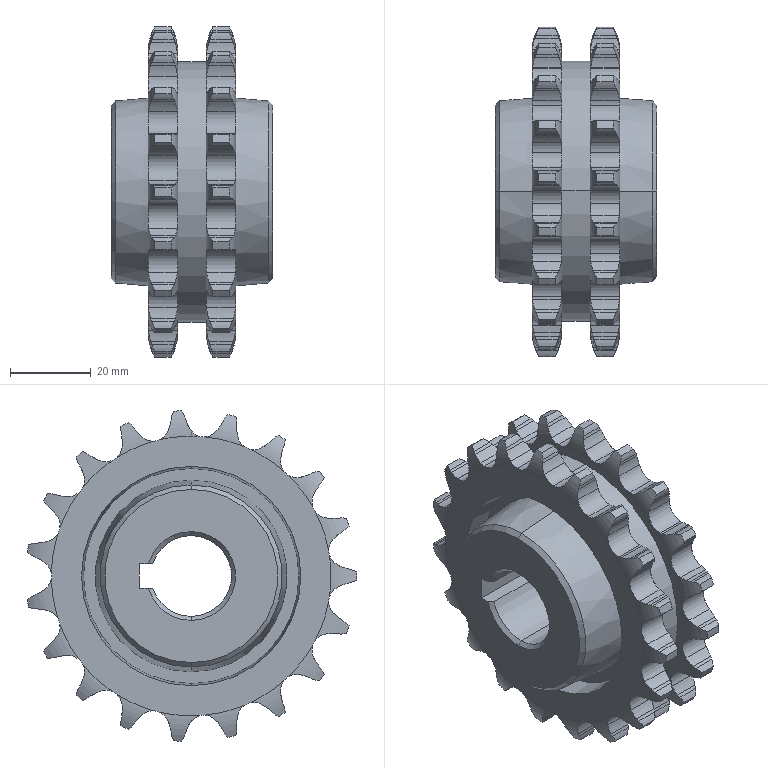Part | SolidWorks | features Cut 2, Revolution 2, Chamfer 1, CirPattern 1, LPattern 1 | 2 solids | 440 faces | box 40 x 81.595 x 81.862 mm | volume 99191 mm3 | cylinder 253 | plane 87 | torus 80 | cone 20 | commonest cylinder face diameters 11.518 x80 20.732 x80 8.06 x48 82 x38 20 x3 54.299 x2